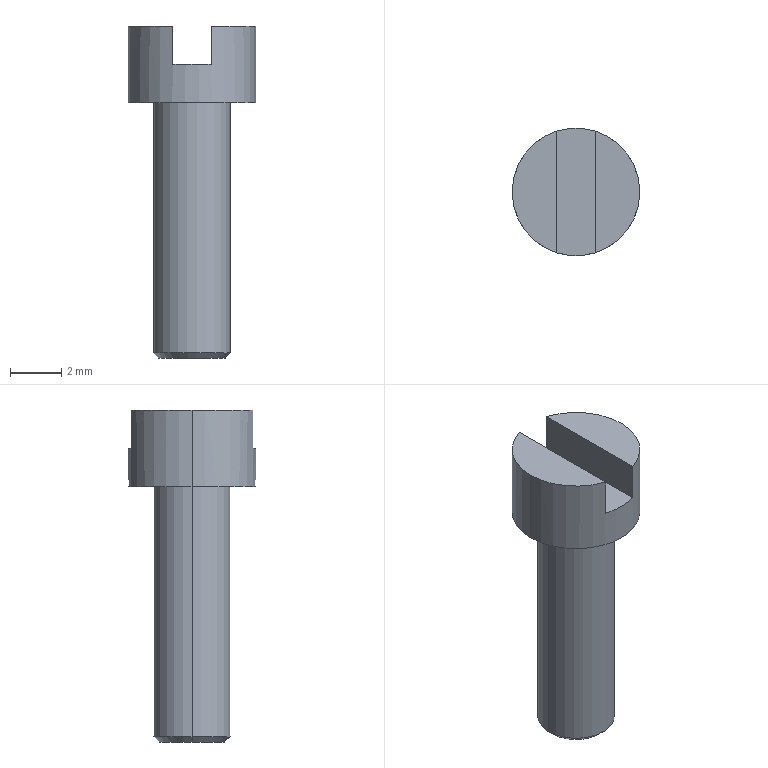Part | SolidWorks | features BaseBody 1 | 1 solid | 13 faces | box 5 x 5 x 13 mm | volume 118.332 mm3 | plane 7 | cylinder 4 | cone 2 | commonest cylinder face diameters 3 x2 5 x2
STEP:
#1=CARTESIAN_POINT('',(1.3,0.,-10.));
#2=VERTEX_POINT('',#1);
#3=CARTESIAN_POINT('',(-1.3,0.,-10.));
#4=VERTEX_POINT('',#3);
#5=CARTESIAN_POINT('',(0.,0.,-10.));
#6=DIRECTION('',(0.,0.,1.));
#7=DIRECTION('',(1.,0.,0.));
#8=AXIS2_PLACEMENT_3D('',#5,#6,#7);
#9=CIRCLE('',#8,1.3);
#10=EDGE_CURVE('',#2,#4,#9,.T.);
#11=ORIENTED_EDGE('',*,*,#10,.T.);
#12=CARTESIAN_POINT('',(-1.5,0.,-9.8));
#13=VERTEX_POINT('',#12);
#14=CARTESIAN_POINT('',(-1.4,0.,-9.9));
#15=DIRECTION('',(-0.7071,0.,0.7071));
#16=VECTOR('',#15,1000.);
#17=LINE('',#14,#16);
#18=EDGE_CURVE('',#4,#13,#17,.T.);
#19=ORIENTED_EDGE('',*,*,#18,.T.);
#20=CARTESIAN_POINT('',(1.5,0.,-9.8));
#21=VERTEX_POINT('',#20);
#22=CARTESIAN_POINT('',(0.,0.,-9.8));
#23=DIRECTION('',(0.,0.,-1.));
#24=DIRECTION('',(1.,0.,0.));
#25=AXIS2_PLACEMENT_3D('',#22,#23,#24);
#26=CIRCLE('',#25,1.5);
#27=EDGE_CURVE('',#13,#21,#26,.T.);
#28=ORIENTED_EDGE('',*,*,#27,.T.);
#29=CARTESIAN_POINT('',(1.4,0.,-9.9));
#30=DIRECTION('',(0.7071,0.,0.7071));
#31=VECTOR('',#30,1000.);
#32=LINE('',#29,#31);
#33=EDGE_CURVE('',#2,#21,#32,.T.);
#34=ORIENTED_EDGE('',*,*,#33,.F.);
#35=EDGE_LOOP('',(#11,#19,#28,#34));
#36=FACE_OUTER_BOUND('',#35,.T.);
#37=CARTESIAN_POINT('',(0.,0.,-9.9));
#38=DIRECTION('',(0.,0.,1.));
#39=DIRECTION('',(1.,0.,0.));
#40=AXIS2_PLACEMENT_3D('',#37,#38,#39);
#41=CONICAL_SURFACE('',#40,1.4,0.7854);
#42=ADVANCED_FACE('',(#36),#41,.T.);
#43=ORIENTED_EDGE('',*,*,#27,.F.);
#44=CARTESIAN_POINT('',(-1.5,0.,0.));
#45=VERTEX_POINT('',#44);
#46=CARTESIAN_POINT('',(-1.5,0.,0.));
#47=DIRECTION('',(0.,0.,1.));
#48=VECTOR('',#47,1000.);
#49=LINE('',#46,#48);
#50=EDGE_CURVE('',#13,#45,#49,.T.);
#51=ORIENTED_EDGE('',*,*,#50,.T.);
#52=CARTESIAN_POINT('',(1.5,0.,0.));
#53=VERTEX_POINT('',#52);
#54=CARTESIAN_POINT('',(0.,0.,0.));
#55=DIRECTION('',(0.,0.,1.));
#56=DIRECTION('',(1.,0.,0.));
#57=AXIS2_PLACEMENT_3D('',#54,#55,#56);
#58=CIRCLE('',#57,1.5);
#59=EDGE_CURVE('',#53,#45,#58,.T.);
#60=ORIENTED_EDGE('',*,*,#59,.F.);
#61=CARTESIAN_POINT('',(1.5,0.,0.));
#62=DIRECTION('',(0.,0.,1.));
#63=VECTOR('',#62,1000.);
#64=LINE('',#61,#63);
#65=EDGE_CURVE('',#21,#53,#64,.T.);
#66=ORIENTED_EDGE('',*,*,#65,.F.);
#67=EDGE_LOOP('',(#43,#51,#60,#66));
#68=FACE_OUTER_BOUND('',#67,.T.);
#69=CARTESIAN_POINT('',(0.,0.,0.));
#70=DIRECTION('',(0.,0.,1.));
#71=DIRECTION('',(1.,0.,0.));
#72=AXIS2_PLACEMENT_3D('',#69,#70,#71);
#73=CYLINDRICAL_SURFACE('',#72,1.5);
#74=ADVANCED_FACE('',(#68),#73,.T.);
#75=CARTESIAN_POINT('',(2.5,0.,3.));
#76=VERTEX_POINT('',#75);
#77=CARTESIAN_POINT('',(0.75,2.385,3.));
#78=VERTEX_POINT('',#77);
#79=CARTESIAN_POINT('',(0.,0.,3.));
#80=DIRECTION('',(0.,0.,1.));
#81=DIRECTION('',(-1.,0.,0.));
#82=AXIS2_PLACEMENT_3D('',#79,#80,#81);
#83=CIRCLE('',#82,2.5);
#84=EDGE_CURVE('',#76,#78,#83,.T.);
#85=ORIENTED_EDGE('',*,*,#84,.F.);
#86=CARTESIAN_POINT('',(2.5,0.,0.));
#87=VERTEX_POINT('',#86);
#88=CARTESIAN_POINT('',(2.5,0.,0.));
#89=DIRECTION('',(0.,0.,-1.));
#90=VECTOR('',#89,1000.);
#91=LINE('',#88,#90);
#92=EDGE_CURVE('',#76,#87,#91,.T.);
#93=ORIENTED_EDGE('',*,*,#92,.T.);
#94=CARTESIAN_POINT('',(-2.5,0.,0.));
#95=VERTEX_POINT('',#94);
#96=CARTESIAN_POINT('',(0.,0.,0.));
#97=DIRECTION('',(0.,0.,-1.));
#98=DIRECTION('',(-1.,0.,0.));
#99=AXIS2_PLACEMENT_3D('',#96,#97,#98);
#100=CIRCLE('',#99,2.5);
#101=EDGE_CURVE('',#95,#87,#100,.T.);
#102=ORIENTED_EDGE('',*,*,#101,.F.);
#103=CARTESIAN_POINT('',(-2.5,0.,3.));
#104=VERTEX_POINT('',#103);
#105=CARTESIAN_POINT('',(-2.5,0.,0.));
#106=DIRECTION('',(0.,0.,-1.));
#107=VECTOR('',#106,1000.);
#108=LINE('',#105,#107);
#109=EDGE_CURVE('',#104,#95,#108,.T.);
#110=ORIENTED_EDGE('',*,*,#109,.F.);
#111=CARTESIAN_POINT('',(-0.75,2.385,3.));
#112=VERTEX_POINT('',#111);
#113=CARTESIAN_POINT('',(0.,0.,3.));
#114=DIRECTION('',(0.,0.,1.));
#115=DIRECTION('',(-1.,0.,0.));
#116=AXIS2_PLACEMENT_3D('',#113,#114,#115);
#117=CIRCLE('',#116,2.5);
#118=EDGE_CURVE('',#112,#104,#117,.T.);
#119=ORIENTED_EDGE('',*,*,#118,.F.);
#120=CARTESIAN_POINT('',(-0.75,2.385,1.5));
#121=VERTEX_POINT('',#120);
#122=CARTESIAN_POINT('',(-0.75,2.385,0.));
#123=DIRECTION('',(0.,0.,-1.));
#124=VECTOR('',#123,1000.);
#125=LINE('',#122,#124);
#126=EDGE_CURVE('',#112,#121,#125,.T.);
#127=ORIENTED_EDGE('',*,*,#126,.T.);
#128=CARTESIAN_POINT('',(0.75,2.385,1.5));
#129=VERTEX_POINT('',#128);
#130=CARTESIAN_POINT('',(0.,0.,1.5));
#131=DIRECTION('',(0.,0.,-1.));
#132=DIRECTION('',(-1.,0.,0.));
#133=AXIS2_PLACEMENT_3D('',#130,#131,#132);
#134=CIRCLE('',#133,2.5);
#135=EDGE_CURVE('',#121,#129,#134,.T.);
#136=ORIENTED_EDGE('',*,*,#135,.T.);
#137=CARTESIAN_POINT('',(0.75,2.385,0.));
#138=DIRECTION('',(0.,0.,1.));
#139=VECTOR('',#138,1000.);
#140=LINE('',#137,#139);
#141=EDGE_CURVE('',#129,#78,#140,.T.);
#142=ORIENTED_EDGE('',*,*,#141,.T.);
#143=EDGE_LOOP('',(#85,#93,#102,#110,#119,#127,#136,#142));
#144=FACE_OUTER_BOUND('',#143,.T.);
#145=CARTESIAN_POINT('',(0.,0.,0.));
#146=DIRECTION('',(0.,0.,-1.));
#147=DIRECTION('',(-1.,0.,0.));
#148=AXIS2_PLACEMENT_3D('',#145,#146,#147);
#149=CYLINDRICAL_SURFACE('',#148,2.5);
#150=ADVANCED_FACE('',(#144),#149,.T.);
#151=ORIENTED_EDGE('',*,*,#10,.F.);
#152=CARTESIAN_POINT('',(0.,0.,-10.));
#153=DIRECTION('',(0.,0.,1.));
#154=DIRECTION('',(1.,0.,0.));
#155=AXIS2_PLACEMENT_3D('',#152,#153,#154);
#156=CIRCLE('',#155,1.3);
#157=EDGE_CURVE('',#4,#2,#156,.T.);
#158=ORIENTED_EDGE('',*,*,#157,.F.);
#159=EDGE_LOOP('',(#151,#158));
#160=FACE_OUTER_BOUND('',#159,.T.);
#161=CARTESIAN_POINT('',(0.,0.,-10.));
#162=DIRECTION('',(0.,0.,1.));
#163=DIRECTION('',(1.,0.,0.));
#164=AXIS2_PLACEMENT_3D('',#161,#162,#163);
#165=PLANE('',#164);
#166=ADVANCED_FACE('',(#160),#165,.F.);
#167=CARTESIAN_POINT('',(-0.75,-2.385,1.5));
#168=VERTEX_POINT('',#167);
#169=CARTESIAN_POINT('',(-0.75,-2.385,3.));
#170=VERTEX_POINT('',#169);
#171=CARTESIAN_POINT('',(-0.75,-2.385,0.));
#172=DIRECTION('',(0.,0.,1.));
#173=VECTOR('',#172,1000.);
#174=LINE('',#171,#173);
#175=EDGE_CURVE('',#168,#170,#174,.T.);
#176=ORIENTED_EDGE('',*,*,#175,.F.);
#177=CARTESIAN_POINT('',(-0.75,-2.5,1.5));
#178=DIRECTION('',(0.,1.,0.));
#179=VECTOR('',#178,1000.);
#180=LINE('',#177,#179);
#181=EDGE_CURVE('',#168,#121,#180,.T.);
#182=ORIENTED_EDGE('',*,*,#181,.T.);
#183=ORIENTED_EDGE('',*,*,#126,.F.);
#184=CARTESIAN_POINT('',(-0.75,-1.25,3.));
#185=DIRECTION('',(0.,1.,0.));
#186=VECTOR('',#185,1000.);
#187=LINE('',#184,#186);
#188=EDGE_CURVE('',#170,#112,#187,.T.);
#189=ORIENTED_EDGE('',*,*,#188,.F.);
#190=EDGE_LOOP('',(#176,#182,#183,#189));
#191=FACE_OUTER_BOUND('',#190,.T.);
#192=CARTESIAN_POINT('',(-0.75,-2.5,3.));
#193=DIRECTION('',(-1.,0.,0.));
#194=DIRECTION('',(0.,1.,0.));
#195=AXIS2_PLACEMENT_3D('',#192,#193,#194);
#196=PLANE('',#195);
#197=ADVANCED_FACE('',(#191),#196,.F.);
#198=CARTESIAN_POINT('',(0.75,-2.385,1.5));
#199=VERTEX_POINT('',#198);
#200=CARTESIAN_POINT('',(0.,0.,1.5));
#201=DIRECTION('',(0.,0.,-1.));
#202=DIRECTION('',(-1.,0.,0.));
#203=AXIS2_PLACEMENT_3D('',#200,#201,#202);
#204=CIRCLE('',#203,2.5);
#205=EDGE_CURVE('',#199,#168,#204,.T.);
#206=ORIENTED_EDGE('',*,*,#205,.F.);
#207=CARTESIAN_POINT('',(0.75,2.5,1.5));
#208=DIRECTION('',(0.,-1.,0.));
#209=VECTOR('',#208,1000.);
#210=LINE('',#207,#209);
#211=EDGE_CURVE('',#129,#199,#210,.T.);
#212=ORIENTED_EDGE('',*,*,#211,.F.);
#213=ORIENTED_EDGE('',*,*,#135,.F.);
#214=ORIENTED_EDGE('',*,*,#181,.F.);
#215=EDGE_LOOP('',(#206,#212,#213,#214));
#216=FACE_OUTER_BOUND('',#215,.T.);
#217=CARTESIAN_POINT('',(0.,0.,1.5));
#218=DIRECTION('',(0.,0.,-1.));
#219=DIRECTION('',(0.,-1.,0.));
#220=AXIS2_PLACEMENT_3D('',#217,#218,#219);
#221=PLANE('',#220);
#222=ADVANCED_FACE('',(#216),#221,.F.);
#223=CARTESIAN_POINT('',(0.75,-2.385,3.));
#224=VERTEX_POINT('',#223);
#225=CARTESIAN_POINT('',(0.75,-2.385,0.));
#226=DIRECTION('',(0.,0.,-1.));
#227=VECTOR('',#226,1000.);
#228=LINE('',#225,#227);
#229=EDGE_CURVE('',#224,#199,#228,.T.);
#230=ORIENTED_EDGE('',*,*,#229,.F.);
#231=CARTESIAN_POINT('',(0.75,1.25,3.));
#232=DIRECTION('',(0.,-1.,0.));
#233=VECTOR('',#232,1000.);
#234=LINE('',#231,#233);
#235=EDGE_CURVE('',#78,#224,#234,.T.);
#236=ORIENTED_EDGE('',*,*,#235,.F.);
#237=ORIENTED_EDGE('',*,*,#141,.F.);
#238=ORIENTED_EDGE('',*,*,#211,.T.);
#239=EDGE_LOOP('',(#230,#236,#237,#238));
#240=FACE_OUTER_BOUND('',#239,.T.);
#241=CARTESIAN_POINT('',(0.75,2.5,3.));
#242=DIRECTION('',(1.,0.,0.));
#243=DIRECTION('',(0.,1.,0.));
#244=AXIS2_PLACEMENT_3D('',#241,#242,#243);
#245=PLANE('',#244);
#246=ADVANCED_FACE('',(#240),#245,.F.);
#247=ORIENTED_EDGE('',*,*,#188,.T.);
#248=ORIENTED_EDGE('',*,*,#118,.T.);
#249=CARTESIAN_POINT('',(0.,0.,3.));
#250=DIRECTION('',(0.,0.,1.));
#251=DIRECTION('',(-1.,0.,0.));
#252=AXIS2_PLACEMENT_3D('',#249,#250,#251);
#253=CIRCLE('',#252,2.5);
#254=EDGE_CURVE('',#104,#170,#253,.T.);
#255=ORIENTED_EDGE('',*,*,#254,.T.);
#256=EDGE_LOOP('',(#247,#248,#255));
#257=FACE_OUTER_BOUND('',#256,.T.);
#258=CARTESIAN_POINT('',(0.,0.,3.));
#259=DIRECTION('',(0.,0.,1.));
#260=DIRECTION('',(1.,0.,0.));
#261=AXIS2_PLACEMENT_3D('',#258,#259,#260);
#262=PLANE('',#261);
#263=ADVANCED_FACE('',(#257),#262,.T.);
#264=ORIENTED_EDGE('',*,*,#59,.T.);
#265=CARTESIAN_POINT('',(0.,0.,0.));
#266=DIRECTION('',(0.,0.,1.));
#267=DIRECTION('',(1.,0.,0.));
#268=AXIS2_PLACEMENT_3D('',#265,#266,#267);
#269=CIRCLE('',#268,1.5);
#270=EDGE_CURVE('',#45,#53,#269,.T.);
#271=ORIENTED_EDGE('',*,*,#270,.T.);
#272=EDGE_LOOP('',(#264,#271));
#273=FACE_BOUND('',#272,.T.);
#274=ORIENTED_EDGE('',*,*,#101,.T.);
#275=CARTESIAN_POINT('',(0.,0.,0.));
#276=DIRECTION('',(0.,0.,-1.));
#277=DIRECTION('',(-1.,0.,0.));
#278=AXIS2_PLACEMENT_3D('',#275,#276,#277);
#279=CIRCLE('',#278,2.5);
#280=EDGE_CURVE('',#87,#95,#279,.T.);
#281=ORIENTED_EDGE('',*,*,#280,.T.);
#282=EDGE_LOOP('',(#274,#281));
#283=FACE_OUTER_BOUND('',#282,.T.);
#284=CARTESIAN_POINT('',(0.,0.,0.));
#285=DIRECTION('',(0.,0.,1.));
#286=DIRECTION('',(1.,0.,0.));
#287=AXIS2_PLACEMENT_3D('',#284,#285,#286);
#288=PLANE('',#287);
#289=ADVANCED_FACE('',(#273,#283),#288,.F.);
#290=ORIENTED_EDGE('',*,*,#235,.T.);
#291=CARTESIAN_POINT('',(0.,0.,3.));
#292=DIRECTION('',(0.,0.,1.));
#293=DIRECTION('',(-1.,0.,0.));
#294=AXIS2_PLACEMENT_3D('',#291,#292,#293);
#295=CIRCLE('',#294,2.5);
#296=EDGE_CURVE('',#224,#76,#295,.T.);
#297=ORIENTED_EDGE('',*,*,#296,.T.);
#298=ORIENTED_EDGE('',*,*,#84,.T.);
#299=EDGE_LOOP('',(#290,#297,#298));
#300=FACE_OUTER_BOUND('',#299,.T.);
#301=CARTESIAN_POINT('',(0.,0.,3.));
#302=DIRECTION('',(0.,0.,1.));
#303=DIRECTION('',(1.,0.,0.));
#304=AXIS2_PLACEMENT_3D('',#301,#302,#303);
#305=PLANE('',#304);
#306=ADVANCED_FACE('',(#300),#305,.T.);
#307=ORIENTED_EDGE('',*,*,#92,.F.);
#308=ORIENTED_EDGE('',*,*,#296,.F.);
#309=ORIENTED_EDGE('',*,*,#229,.T.);
#310=ORIENTED_EDGE('',*,*,#205,.T.);
#311=ORIENTED_EDGE('',*,*,#175,.T.);
#312=ORIENTED_EDGE('',*,*,#254,.F.);
#313=ORIENTED_EDGE('',*,*,#109,.T.);
#314=ORIENTED_EDGE('',*,*,#280,.F.);
#315=EDGE_LOOP('',(#307,#308,#309,#310,#311,#312,#313,#314));
#316=FACE_OUTER_BOUND('',#315,.T.);
#317=CARTESIAN_POINT('',(0.,0.,0.));
#318=DIRECTION('',(0.,0.,-1.));
#319=DIRECTION('',(-1.,0.,0.));
#320=AXIS2_PLACEMENT_3D('',#317,#318,#319);
#321=CYLINDRICAL_SURFACE('',#320,2.5);
#322=ADVANCED_FACE('',(#316),#321,.T.);
#323=ORIENTED_EDGE('',*,*,#50,.F.);
#324=CARTESIAN_POINT('',(0.,0.,-9.8));
#325=DIRECTION('',(0.,0.,-1.));
#326=DIRECTION('',(1.,0.,0.));
#327=AXIS2_PLACEMENT_3D('',#324,#325,#326);
#328=CIRCLE('',#327,1.5);
#329=EDGE_CURVE('',#21,#13,#328,.T.);
#330=ORIENTED_EDGE('',*,*,#329,.F.);
#331=ORIENTED_EDGE('',*,*,#65,.T.);
#332=ORIENTED_EDGE('',*,*,#270,.F.);
#333=EDGE_LOOP('',(#323,#330,#331,#332));
#334=FACE_OUTER_BOUND('',#333,.T.);
#335=CARTESIAN_POINT('',(0.,0.,0.));
#336=DIRECTION('',(0.,0.,1.));
#337=DIRECTION('',(1.,0.,0.));
#338=AXIS2_PLACEMENT_3D('',#335,#336,#337);
#339=CYLINDRICAL_SURFACE('',#338,1.5);
#340=ADVANCED_FACE('',(#334),#339,.T.);
#341=ORIENTED_EDGE('',*,*,#18,.F.);
#342=ORIENTED_EDGE('',*,*,#157,.T.);
#343=ORIENTED_EDGE('',*,*,#33,.T.);
#344=ORIENTED_EDGE('',*,*,#329,.T.);
#345=EDGE_LOOP('',(#341,#342,#343,#344));
#346=FACE_OUTER_BOUND('',#345,.T.);
#347=CARTESIAN_POINT('',(0.,0.,-9.9));
#348=DIRECTION('',(0.,0.,1.));
#349=DIRECTION('',(1.,0.,0.));
#350=AXIS2_PLACEMENT_3D('',#347,#348,#349);
#351=CONICAL_SURFACE('',#350,1.4,0.7854);
#352=ADVANCED_FACE('',(#346),#351,.T.);
#353=CLOSED_SHELL('',(#42,#74,#150,#166,#197,#222,#246,#263,#289,#306,#322,#340,#352));
#354=MANIFOLD_SOLID_BREP('',#353);
#355=CARTESIAN_POINT('',(0.,0.,0.));
#356=DIRECTION('',(0.,0.,1.));
#357=DIRECTION('',(1.,0.,0.));
#358=AXIS2_PLACEMENT_3D('',#355,#356,#357);
#359=(LENGTH_UNIT()NAMED_UNIT(*)SI_UNIT(.MILLI.,.METRE.));
#360=UNCERTAINTY_MEASURE_WITH_UNIT(LENGTH_MEASURE(0.00001),#359,'','');
#361=(NAMED_UNIT(*)PLANE_ANGLE_UNIT()SI_UNIT($,.RADIAN.));
#362=(NAMED_UNIT(*)SI_UNIT($,.STERADIAN.)SOLID_ANGLE_UNIT());
#363=(GEOMETRIC_REPRESENTATION_CONTEXT(3)GLOBAL_UNCERTAINTY_ASSIGNED_CONTEXT((#360))GLOBAL_UNIT_ASSIGNED_CONTEXT((#359,#361,#362))REPRESENTATION_CONTEXT('',''));
#364=ADVANCED_BREP_SHAPE_REPRESENTATION('',(#354,#358),#363);